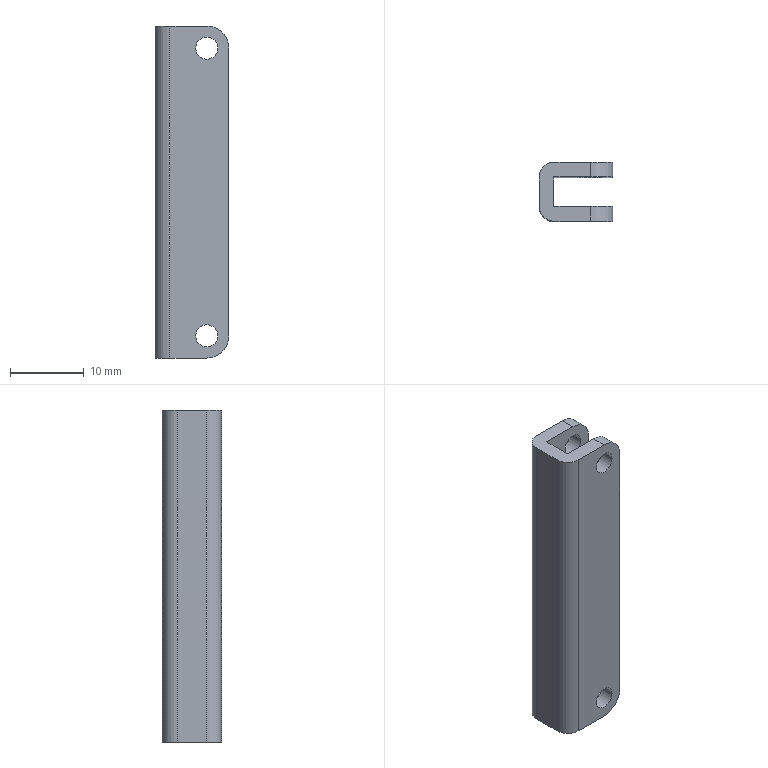Part | SolidWorks | features Extrusion 1, Fillet 1, ICE 1 | 1 solid | 24 faces | box 10 x 8 x 45 mm | volume 2011 mm3 | cylinder 14 | plane 10 | commonest cylinder face diameters 3 x8 6 x4 4 x2
STEP:
#1=CARTESIAN_POINT('',(-4.5,4.,3.));
#2=VERTEX_POINT('',#1);
#3=CARTESIAN_POINT('',(-1.5,4.,3.));
#4=VERTEX_POINT('',#3);
#5=CARTESIAN_POINT('',(-3.,4.,3.));
#6=DIRECTION('',(0.,-1.,0.));
#7=DIRECTION('',(1.,0.,0.));
#8=AXIS2_PLACEMENT_3D('',#5,#6,#7);
#9=CIRCLE('',#8,1.5);
#10=EDGE_CURVE('',#2,#4,#9,.T.);
#11=ORIENTED_EDGE('',*,*,#10,.F.);
#12=CARTESIAN_POINT('',(-4.5,2.,3.));
#13=VERTEX_POINT('',#12);
#14=CARTESIAN_POINT('',(-4.5,4.,3.));
#15=DIRECTION('',(0.,-1.,0.));
#16=VECTOR('',#15,1000.);
#17=LINE('',#14,#16);
#18=EDGE_CURVE('',#2,#13,#17,.T.);
#19=ORIENTED_EDGE('',*,*,#18,.T.);
#20=CARTESIAN_POINT('',(-1.5,2.,3.));
#21=VERTEX_POINT('',#20);
#22=CARTESIAN_POINT('',(-3.,2.,3.));
#23=DIRECTION('',(0.,1.,0.));
#24=DIRECTION('',(-1.,0.,0.));
#25=AXIS2_PLACEMENT_3D('',#22,#23,#24);
#26=CIRCLE('',#25,1.5);
#27=EDGE_CURVE('',#21,#13,#26,.T.);
#28=ORIENTED_EDGE('',*,*,#27,.F.);
#29=CARTESIAN_POINT('',(-1.5,4.,3.));
#30=DIRECTION('',(0.,-1.,0.));
#31=VECTOR('',#30,1000.);
#32=LINE('',#29,#31);
#33=EDGE_CURVE('',#4,#21,#32,.T.);
#34=ORIENTED_EDGE('',*,*,#33,.F.);
#35=EDGE_LOOP('',(#11,#19,#28,#34));
#36=FACE_OUTER_BOUND('',#35,.T.);
#37=CARTESIAN_POINT('',(-3.,4.,3.));
#38=DIRECTION('',(0.,-1.,0.));
#39=DIRECTION('',(1.,0.,0.));
#40=AXIS2_PLACEMENT_3D('',#37,#38,#39);
#41=CYLINDRICAL_SURFACE('',#40,1.5);
#42=ADVANCED_FACE('',(#36),#41,.F.);
#43=CARTESIAN_POINT('',(-4.5,4.,42.));
#44=VERTEX_POINT('',#43);
#45=CARTESIAN_POINT('',(-1.5,4.,42.));
#46=VERTEX_POINT('',#45);
#47=CARTESIAN_POINT('',(-3.,4.,42.));
#48=DIRECTION('',(0.,-1.,0.));
#49=DIRECTION('',(1.,0.,0.));
#50=AXIS2_PLACEMENT_3D('',#47,#48,#49);
#51=CIRCLE('',#50,1.5);
#52=EDGE_CURVE('',#44,#46,#51,.T.);
#53=ORIENTED_EDGE('',*,*,#52,.F.);
#54=CARTESIAN_POINT('',(-4.5,2.,42.));
#55=VERTEX_POINT('',#54);
#56=CARTESIAN_POINT('',(-4.5,4.,42.));
#57=DIRECTION('',(0.,-1.,0.));
#58=VECTOR('',#57,1000.);
#59=LINE('',#56,#58);
#60=EDGE_CURVE('',#44,#55,#59,.T.);
#61=ORIENTED_EDGE('',*,*,#60,.T.);
#62=CARTESIAN_POINT('',(-1.5,2.,42.));
#63=VERTEX_POINT('',#62);
#64=CARTESIAN_POINT('',(-3.,2.,42.));
#65=DIRECTION('',(0.,1.,0.));
#66=DIRECTION('',(-1.,0.,0.));
#67=AXIS2_PLACEMENT_3D('',#64,#65,#66);
#68=CIRCLE('',#67,1.5);
#69=EDGE_CURVE('',#63,#55,#68,.T.);
#70=ORIENTED_EDGE('',*,*,#69,.F.);
#71=CARTESIAN_POINT('',(-1.5,4.,42.));
#72=DIRECTION('',(0.,-1.,0.));
#73=VECTOR('',#72,1000.);
#74=LINE('',#71,#73);
#75=EDGE_CURVE('',#46,#63,#74,.T.);
#76=ORIENTED_EDGE('',*,*,#75,.F.);
#77=EDGE_LOOP('',(#53,#61,#70,#76));
#78=FACE_OUTER_BOUND('',#77,.T.);
#79=CARTESIAN_POINT('',(-3.,4.,42.));
#80=DIRECTION('',(0.,-1.,0.));
#81=DIRECTION('',(1.,0.,0.));
#82=AXIS2_PLACEMENT_3D('',#79,#80,#81);
#83=CYLINDRICAL_SURFACE('',#82,1.5);
#84=ADVANCED_FACE('',(#78),#83,.F.);
#85=CARTESIAN_POINT('',(-4.5,-2.,3.));
#86=VERTEX_POINT('',#85);
#87=CARTESIAN_POINT('',(-1.5,-2.,3.));
#88=VERTEX_POINT('',#87);
#89=CARTESIAN_POINT('',(-3.,-2.,3.));
#90=DIRECTION('',(0.,-1.,0.));
#91=DIRECTION('',(1.,0.,0.));
#92=AXIS2_PLACEMENT_3D('',#89,#90,#91);
#93=CIRCLE('',#92,1.5);
#94=EDGE_CURVE('',#86,#88,#93,.T.);
#95=ORIENTED_EDGE('',*,*,#94,.F.);
#96=CARTESIAN_POINT('',(-4.5,-4.,3.));
#97=VERTEX_POINT('',#96);
#98=CARTESIAN_POINT('',(-4.5,4.,3.));
#99=DIRECTION('',(0.,-1.,0.));
#100=VECTOR('',#99,1000.);
#101=LINE('',#98,#100);
#102=EDGE_CURVE('',#86,#97,#101,.T.);
#103=ORIENTED_EDGE('',*,*,#102,.T.);
#104=CARTESIAN_POINT('',(-1.5,-4.,3.));
#105=VERTEX_POINT('',#104);
#106=CARTESIAN_POINT('',(-3.,-4.,3.));
#107=DIRECTION('',(0.,-1.,0.));
#108=DIRECTION('',(1.,0.,0.));
#109=AXIS2_PLACEMENT_3D('',#106,#107,#108);
#110=CIRCLE('',#109,1.5);
#111=EDGE_CURVE('',#97,#105,#110,.T.);
#112=ORIENTED_EDGE('',*,*,#111,.T.);
#113=CARTESIAN_POINT('',(-1.5,4.,3.));
#114=DIRECTION('',(0.,-1.,0.));
#115=VECTOR('',#114,1000.);
#116=LINE('',#113,#115);
#117=EDGE_CURVE('',#88,#105,#116,.T.);
#118=ORIENTED_EDGE('',*,*,#117,.F.);
#119=EDGE_LOOP('',(#95,#103,#112,#118));
#120=FACE_OUTER_BOUND('',#119,.T.);
#121=CARTESIAN_POINT('',(-3.,4.,3.));
#122=DIRECTION('',(0.,-1.,0.));
#123=DIRECTION('',(1.,0.,0.));
#124=AXIS2_PLACEMENT_3D('',#121,#122,#123);
#125=CYLINDRICAL_SURFACE('',#124,1.5);
#126=ADVANCED_FACE('',(#120),#125,.F.);
#127=CARTESIAN_POINT('',(-4.5,-2.,42.));
#128=VERTEX_POINT('',#127);
#129=CARTESIAN_POINT('',(-1.5,-2.,42.));
#130=VERTEX_POINT('',#129);
#131=CARTESIAN_POINT('',(-3.,-2.,42.));
#132=DIRECTION('',(0.,-1.,0.));
#133=DIRECTION('',(1.,0.,0.));
#134=AXIS2_PLACEMENT_3D('',#131,#132,#133);
#135=CIRCLE('',#134,1.5);
#136=EDGE_CURVE('',#128,#130,#135,.T.);
#137=ORIENTED_EDGE('',*,*,#136,.F.);
#138=CARTESIAN_POINT('',(-4.5,-4.,42.));
#139=VERTEX_POINT('',#138);
#140=CARTESIAN_POINT('',(-4.5,4.,42.));
#141=DIRECTION('',(0.,-1.,0.));
#142=VECTOR('',#141,1000.);
#143=LINE('',#140,#142);
#144=EDGE_CURVE('',#128,#139,#143,.T.);
#145=ORIENTED_EDGE('',*,*,#144,.T.);
#146=CARTESIAN_POINT('',(-1.5,-4.,42.));
#147=VERTEX_POINT('',#146);
#148=CARTESIAN_POINT('',(-3.,-4.,42.));
#149=DIRECTION('',(0.,-1.,0.));
#150=DIRECTION('',(1.,0.,0.));
#151=AXIS2_PLACEMENT_3D('',#148,#149,#150);
#152=CIRCLE('',#151,1.5);
#153=EDGE_CURVE('',#139,#147,#152,.T.);
#154=ORIENTED_EDGE('',*,*,#153,.T.);
#155=CARTESIAN_POINT('',(-1.5,4.,42.));
#156=DIRECTION('',(0.,-1.,0.));
#157=VECTOR('',#156,1000.);
#158=LINE('',#155,#157);
#159=EDGE_CURVE('',#130,#147,#158,.T.);
#160=ORIENTED_EDGE('',*,*,#159,.F.);
#161=EDGE_LOOP('',(#137,#145,#154,#160));
#162=FACE_OUTER_BOUND('',#161,.T.);
#163=CARTESIAN_POINT('',(-3.,4.,42.));
#164=DIRECTION('',(0.,-1.,0.));
#165=DIRECTION('',(1.,0.,0.));
#166=AXIS2_PLACEMENT_3D('',#163,#164,#165);
#167=CYLINDRICAL_SURFACE('',#166,1.5);
#168=ADVANCED_FACE('',(#162),#167,.F.);
#169=CARTESIAN_POINT('',(0.,-2.,42.));
#170=VERTEX_POINT('',#169);
#171=CARTESIAN_POINT('',(0.,-2.,3.));
#172=VERTEX_POINT('',#171);
#173=CARTESIAN_POINT('',(0.,-2.,45.));
#174=DIRECTION('',(0.,0.,-1.));
#175=VECTOR('',#174,1000.);
#176=LINE('',#173,#175);
#177=EDGE_CURVE('',#170,#172,#176,.T.);
#178=ORIENTED_EDGE('',*,*,#177,.F.);
#179=CARTESIAN_POINT('',(0.,-4.,42.));
#180=VERTEX_POINT('',#179);
#181=CARTESIAN_POINT('',(0.,-4.,42.));
#182=DIRECTION('',(0.,-1.,0.));
#183=VECTOR('',#182,1000.);
#184=LINE('',#181,#183);
#185=EDGE_CURVE('',#170,#180,#184,.T.);
#186=ORIENTED_EDGE('',*,*,#185,.T.);
#187=CARTESIAN_POINT('',(0.,-4.,3.));
#188=VERTEX_POINT('',#187);
#189=CARTESIAN_POINT('',(0.,-4.,45.));
#190=DIRECTION('',(0.,0.,-1.));
#191=VECTOR('',#190,1000.);
#192=LINE('',#189,#191);
#193=EDGE_CURVE('',#180,#188,#192,.T.);
#194=ORIENTED_EDGE('',*,*,#193,.T.);
#195=CARTESIAN_POINT('',(0.,-4.,3.));
#196=DIRECTION('',(0.,1.,0.));
#197=VECTOR('',#196,1000.);
#198=LINE('',#195,#197);
#199=EDGE_CURVE('',#188,#172,#198,.T.);
#200=ORIENTED_EDGE('',*,*,#199,.T.);
#201=EDGE_LOOP('',(#178,#186,#194,#200));
#202=FACE_OUTER_BOUND('',#201,.T.);
#203=CARTESIAN_POINT('',(0.,-4.,45.));
#204=DIRECTION('',(-1.,0.,0.));
#205=DIRECTION('',(0.,-1.,0.));
#206=AXIS2_PLACEMENT_3D('',#203,#204,#205);
#207=PLANE('',#206);
#208=ADVANCED_FACE('',(#202),#207,.F.);
#209=CARTESIAN_POINT('',(-3.,-2.,3.));
#210=DIRECTION('',(0.,-1.,0.));
#211=DIRECTION('',(1.,0.,0.));
#212=AXIS2_PLACEMENT_3D('',#209,#210,#211);
#213=CIRCLE('',#212,1.5);
#214=EDGE_CURVE('',#88,#86,#213,.T.);
#215=ORIENTED_EDGE('',*,*,#214,.T.);
#216=ORIENTED_EDGE('',*,*,#94,.T.);
#217=EDGE_LOOP('',(#215,#216));
#218=FACE_BOUND('',#217,.T.);
#219=CARTESIAN_POINT('',(-3.,-2.,42.));
#220=DIRECTION('',(0.,-1.,0.));
#221=DIRECTION('',(1.,0.,0.));
#222=AXIS2_PLACEMENT_3D('',#219,#220,#221);
#223=CIRCLE('',#222,1.5);
#224=EDGE_CURVE('',#130,#128,#223,.T.);
#225=ORIENTED_EDGE('',*,*,#224,.T.);
#226=ORIENTED_EDGE('',*,*,#136,.T.);
#227=EDGE_LOOP('',(#225,#226));
#228=FACE_BOUND('',#227,.T.);
#229=CARTESIAN_POINT('',(-3.,-2.,45.));
#230=VERTEX_POINT('',#229);
#231=CARTESIAN_POINT('',(-8.,-2.,45.));
#232=VERTEX_POINT('',#231);
#233=CARTESIAN_POINT('',(-8.,-2.,45.));
#234=DIRECTION('',(-1.,0.,0.));
#235=VECTOR('',#234,1000.);
#236=LINE('',#233,#235);
#237=EDGE_CURVE('',#230,#232,#236,.T.);
#238=ORIENTED_EDGE('',*,*,#237,.F.);
#239=CARTESIAN_POINT('',(-3.,-2.,42.));
#240=DIRECTION('',(0.,1.,0.));
#241=DIRECTION('',(1.,0.,0.));
#242=AXIS2_PLACEMENT_3D('',#239,#240,#241);
#243=CIRCLE('',#242,3.);
#244=EDGE_CURVE('',#230,#170,#243,.T.);
#245=ORIENTED_EDGE('',*,*,#244,.T.);
#246=ORIENTED_EDGE('',*,*,#177,.T.);
#247=CARTESIAN_POINT('',(-3.,-2.,0.));
#248=VERTEX_POINT('',#247);
#249=CARTESIAN_POINT('',(-3.,-2.,3.));
#250=DIRECTION('',(0.,1.,0.));
#251=DIRECTION('',(1.,0.,0.));
#252=AXIS2_PLACEMENT_3D('',#249,#250,#251);
#253=CIRCLE('',#252,3.);
#254=EDGE_CURVE('',#172,#248,#253,.T.);
#255=ORIENTED_EDGE('',*,*,#254,.T.);
#256=CARTESIAN_POINT('',(-8.,-2.,0.));
#257=VERTEX_POINT('',#256);
#258=CARTESIAN_POINT('',(-8.,-2.,0.));
#259=DIRECTION('',(-1.,0.,0.));
#260=VECTOR('',#259,1000.);
#261=LINE('',#258,#260);
#262=EDGE_CURVE('',#248,#257,#261,.T.);
#263=ORIENTED_EDGE('',*,*,#262,.T.);
#264=CARTESIAN_POINT('',(-8.,-2.,45.));
#265=DIRECTION('',(0.,0.,-1.));
#266=VECTOR('',#265,1000.);
#267=LINE('',#264,#266);
#268=EDGE_CURVE('',#232,#257,#267,.T.);
#269=ORIENTED_EDGE('',*,*,#268,.F.);
#270=EDGE_LOOP('',(#238,#245,#246,#255,#263,#269));
#271=FACE_OUTER_BOUND('',#270,.T.);
#272=CARTESIAN_POINT('',(-8.,-2.,45.));
#273=DIRECTION('',(0.,-1.,0.));
#274=DIRECTION('',(1.,0.,0.));
#275=AXIS2_PLACEMENT_3D('',#272,#273,#274);
#276=PLANE('',#275);
#277=ADVANCED_FACE('',(#218,#228,#271),#276,.F.);
#278=CARTESIAN_POINT('',(-8.,2.,0.));
#279=VERTEX_POINT('',#278);
#280=CARTESIAN_POINT('',(-8.,2.,0.));
#281=DIRECTION('',(0.,1.,0.));
#282=VECTOR('',#281,1000.);
#283=LINE('',#280,#282);
#284=EDGE_CURVE('',#257,#279,#283,.T.);
#285=ORIENTED_EDGE('',*,*,#284,.T.);
#286=CARTESIAN_POINT('',(-8.,2.,45.));
#287=VERTEX_POINT('',#286);
#288=CARTESIAN_POINT('',(-8.,2.,45.));
#289=DIRECTION('',(0.,0.,-1.));
#290=VECTOR('',#289,1000.);
#291=LINE('',#288,#290);
#292=EDGE_CURVE('',#287,#279,#291,.T.);
#293=ORIENTED_EDGE('',*,*,#292,.F.);
#294=CARTESIAN_POINT('',(-8.,2.,45.));
#295=DIRECTION('',(0.,1.,0.));
#296=VECTOR('',#295,1000.);
#297=LINE('',#294,#296);
#298=EDGE_CURVE('',#232,#287,#297,.T.);
#299=ORIENTED_EDGE('',*,*,#298,.F.);
#300=ORIENTED_EDGE('',*,*,#268,.T.);
#301=EDGE_LOOP('',(#285,#293,#299,#300));
#302=FACE_OUTER_BOUND('',#301,.T.);
#303=CARTESIAN_POINT('',(-8.,2.,45.));
#304=DIRECTION('',(-1.,0.,0.));
#305=DIRECTION('',(0.,0.,1.));
#306=AXIS2_PLACEMENT_3D('',#303,#304,#305);
#307=PLANE('',#306);
#308=ADVANCED_FACE('',(#302),#307,.F.);
#309=ORIENTED_EDGE('',*,*,#27,.T.);
#310=CARTESIAN_POINT('',(-3.,2.,3.));
#311=DIRECTION('',(0.,1.,0.));
#312=DIRECTION('',(-1.,0.,0.));
#313=AXIS2_PLACEMENT_3D('',#310,#311,#312);
#314=CIRCLE('',#313,1.5);
#315=EDGE_CURVE('',#13,#21,#314,.T.);
#316=ORIENTED_EDGE('',*,*,#315,.T.);
#317=EDGE_LOOP('',(#309,#316));
#318=FACE_BOUND('',#317,.T.);
#319=ORIENTED_EDGE('',*,*,#69,.T.);
#320=CARTESIAN_POINT('',(-3.,2.,42.));
#321=DIRECTION('',(0.,1.,0.));
#322=DIRECTION('',(-1.,0.,0.));
#323=AXIS2_PLACEMENT_3D('',#320,#321,#322);
#324=CIRCLE('',#323,1.5);
#325=EDGE_CURVE('',#55,#63,#324,.T.);
#326=ORIENTED_EDGE('',*,*,#325,.T.);
#327=EDGE_LOOP('',(#319,#326));
#328=FACE_BOUND('',#327,.T.);
#329=CARTESIAN_POINT('',(0.,2.,42.));
#330=VERTEX_POINT('',#329);
#331=CARTESIAN_POINT('',(0.,2.,3.));
#332=VERTEX_POINT('',#331);
#333=CARTESIAN_POINT('',(0.,2.,45.));
#334=DIRECTION('',(0.,0.,-1.));
#335=VECTOR('',#334,1000.);
#336=LINE('',#333,#335);
#337=EDGE_CURVE('',#330,#332,#336,.T.);
#338=ORIENTED_EDGE('',*,*,#337,.F.);
#339=CARTESIAN_POINT('',(-3.,2.,45.));
#340=VERTEX_POINT('',#339);
#341=CARTESIAN_POINT('',(-3.,2.,42.));
#342=DIRECTION('',(0.,-1.,0.));
#343=DIRECTION('',(-1.,0.,0.));
#344=AXIS2_PLACEMENT_3D('',#341,#342,#343);
#345=CIRCLE('',#344,3.);
#346=EDGE_CURVE('',#330,#340,#345,.T.);
#347=ORIENTED_EDGE('',*,*,#346,.T.);
#348=CARTESIAN_POINT('',(-8.,2.,45.));
#349=DIRECTION('',(1.,0.,0.));
#350=VECTOR('',#349,1000.);
#351=LINE('',#348,#350);
#352=EDGE_CURVE('',#287,#340,#351,.T.);
#353=ORIENTED_EDGE('',*,*,#352,.F.);
#354=ORIENTED_EDGE('',*,*,#292,.T.);
#355=CARTESIAN_POINT('',(-3.,2.,0.));
#356=VERTEX_POINT('',#355);
#357=CARTESIAN_POINT('',(-8.,2.,0.));
#358=DIRECTION('',(1.,0.,0.));
#359=VECTOR('',#358,1000.);
#360=LINE('',#357,#359);
#361=EDGE_CURVE('',#279,#356,#360,.T.);
#362=ORIENTED_EDGE('',*,*,#361,.T.);
#363=CARTESIAN_POINT('',(-3.,2.,3.));
#364=DIRECTION('',(0.,-1.,0.));
#365=DIRECTION('',(-1.,0.,0.));
#366=AXIS2_PLACEMENT_3D('',#363,#364,#365);
#367=CIRCLE('',#366,3.);
#368=EDGE_CURVE('',#356,#332,#367,.T.);
#369=ORIENTED_EDGE('',*,*,#368,.T.);
#370=EDGE_LOOP('',(#338,#347,#353,#354,#362,#369));
#371=FACE_OUTER_BOUND('',#370,.T.);
#372=CARTESIAN_POINT('',(-8.,2.,45.));
#373=DIRECTION('',(0.,1.,0.));
#374=DIRECTION('',(-1.,0.,0.));
#375=AXIS2_PLACEMENT_3D('',#372,#373,#374);
#376=PLANE('',#375);
#377=ADVANCED_FACE('',(#318,#328,#371),#376,.F.);
#378=CARTESIAN_POINT('',(0.,4.,42.));
#379=VERTEX_POINT('',#378);
#380=CARTESIAN_POINT('',(0.,4.,3.));
#381=VERTEX_POINT('',#380);
#382=CARTESIAN_POINT('',(0.,4.,45.));
#383=DIRECTION('',(0.,0.,-1.));
#384=VECTOR('',#383,1000.);
#385=LINE('',#382,#384);
#386=EDGE_CURVE('',#379,#381,#385,.T.);
#387=ORIENTED_EDGE('',*,*,#386,.F.);
#388=CARTESIAN_POINT('',(0.,2.,42.));
#389=DIRECTION('',(0.,-1.,0.));
#390=VECTOR('',#389,1000.);
#391=LINE('',#388,#390);
#392=EDGE_CURVE('',#379,#330,#391,.T.);
#393=ORIENTED_EDGE('',*,*,#392,.T.);
#394=ORIENTED_EDGE('',*,*,#337,.T.);
#395=CARTESIAN_POINT('',(0.,4.,3.));
#396=DIRECTION('',(0.,1.,0.));
#397=VECTOR('',#396,1000.);
#398=LINE('',#395,#397);
#399=EDGE_CURVE('',#332,#381,#398,.T.);
#400=ORIENTED_EDGE('',*,*,#399,.T.);
#401=EDGE_LOOP('',(#387,#393,#394,#400));
#402=FACE_OUTER_BOUND('',#401,.T.);
#403=CARTESIAN_POINT('',(0.,4.,45.));
#404=DIRECTION('',(-1.,0.,0.));
#405=DIRECTION('',(0.,-1.,0.));
#406=AXIS2_PLACEMENT_3D('',#403,#404,#405);
#407=PLANE('',#406);
#408=ADVANCED_FACE('',(#402),#407,.F.);
#409=CARTESIAN_POINT('',(-3.,4.,3.));
#410=DIRECTION('',(0.,-1.,0.));
#411=DIRECTION('',(1.,0.,0.));
#412=AXIS2_PLACEMENT_3D('',#409,#410,#411);
#413=CIRCLE('',#412,1.5);
#414=EDGE_CURVE('',#4,#2,#413,.T.);
#415=ORIENTED_EDGE('',*,*,#414,.T.);
#416=ORIENTED_EDGE('',*,*,#10,.T.);
#417=EDGE_LOOP('',(#415,#416));
#418=FACE_BOUND('',#417,.T.);
#419=CARTESIAN_POINT('',(-3.,4.,42.));
#420=DIRECTION('',(0.,-1.,0.));
#421=DIRECTION('',(1.,0.,0.));
#422=AXIS2_PLACEMENT_3D('',#419,#420,#421);
#423=CIRCLE('',#422,1.5);
#424=EDGE_CURVE('',#46,#44,#423,.T.);
#425=ORIENTED_EDGE('',*,*,#424,.T.);
#426=ORIENTED_EDGE('',*,*,#52,.T.);
#427=EDGE_LOOP('',(#425,#426));
#428=FACE_BOUND('',#427,.T.);
#429=CARTESIAN_POINT('',(-3.,4.,45.));
#430=VERTEX_POINT('',#429);
#431=CARTESIAN_POINT('',(-8.,4.,45.));
#432=VERTEX_POINT('',#431);
#433=CARTESIAN_POINT('',(-8.,4.,45.));
#434=DIRECTION('',(-1.,0.,0.));
#435=VECTOR('',#434,1000.);
#436=LINE('',#433,#435);
#437=EDGE_CURVE('',#430,#432,#436,.T.);
#438=ORIENTED_EDGE('',*,*,#437,.F.);
#439=CARTESIAN_POINT('',(-3.,4.,42.));
#440=DIRECTION('',(0.,1.,0.));
#441=DIRECTION('',(1.,0.,0.));
#442=AXIS2_PLACEMENT_3D('',#439,#440,#441);
#443=CIRCLE('',#442,3.);
#444=EDGE_CURVE('',#430,#379,#443,.T.);
#445=ORIENTED_EDGE('',*,*,#444,.T.);
#446=ORIENTED_EDGE('',*,*,#386,.T.);
#447=CARTESIAN_POINT('',(-3.,4.,0.));
#448=VERTEX_POINT('',#447);
#449=CARTESIAN_POINT('',(-3.,4.,3.));
#450=DIRECTION('',(0.,1.,0.));
#451=DIRECTION('',(1.,0.,0.));
#452=AXIS2_PLACEMENT_3D('',#449,#450,#451);
#453=CIRCLE('',#452,3.);
#454=EDGE_CURVE('',#381,#448,#453,.T.);
#455=ORIENTED_EDGE('',*,*,#454,.T.);
#456=CARTESIAN_POINT('',(-8.,4.,0.));
#457=VERTEX_POINT('',#456);
#458=CARTESIAN_POINT('',(-8.,4.,0.));
#459=DIRECTION('',(-1.,0.,0.));
#460=VECTOR('',#459,1000.);
#461=LINE('',#458,#460);
#462=EDGE_CURVE('',#448,#457,#461,.T.);
#463=ORIENTED_EDGE('',*,*,#462,.T.);
#464=CARTESIAN_POINT('',(-8.,4.,45.));
#465=DIRECTION('',(0.,0.,-1.));
#466=VECTOR('',#465,1000.);
#467=LINE('',#464,#466);
#468=EDGE_CURVE('',#432,#457,#467,.T.);
#469=ORIENTED_EDGE('',*,*,#468,.F.);
#470=EDGE_LOOP('',(#438,#445,#446,#455,#463,#469));
#471=FACE_OUTER_BOUND('',#470,.T.);
#472=CARTESIAN_POINT('',(-8.,4.,45.));
#473=DIRECTION('',(0.,-1.,0.));
#474=DIRECTION('',(1.,0.,0.));
#475=AXIS2_PLACEMENT_3D('',#472,#473,#474);
#476=PLANE('',#475);
#477=ADVANCED_FACE('',(#418,#428,#471),#476,.F.);
#478=CARTESIAN_POINT('',(-10.,2.,0.));
#479=VERTEX_POINT('',#478);
#480=CARTESIAN_POINT('',(-8.,2.,0.));
#481=DIRECTION('',(0.,0.,1.));
#482=DIRECTION('',(1.,0.,0.));
#483=AXIS2_PLACEMENT_3D('',#480,#481,#482);
#484=CIRCLE('',#483,2.);
#485=EDGE_CURVE('',#457,#479,#484,.T.);
#486=ORIENTED_EDGE('',*,*,#485,.T.);
#487=CARTESIAN_POINT('',(-10.,2.,45.));
#488=VERTEX_POINT('',#487);
#489=CARTESIAN_POINT('',(-10.,2.,45.));
#490=DIRECTION('',(0.,0.,-1.));
#491=VECTOR('',#490,1000.);
#492=LINE('',#489,#491);
#493=EDGE_CURVE('',#488,#479,#492,.T.);
#494=ORIENTED_EDGE('',*,*,#493,.F.);
#495=CARTESIAN_POINT('',(-8.,2.,45.));
#496=DIRECTION('',(0.,0.,1.));
#497=DIRECTION('',(1.,0.,0.));
#498=AXIS2_PLACEMENT_3D('',#495,#496,#497);
#499=CIRCLE('',#498,2.);
#500=EDGE_CURVE('',#432,#488,#499,.T.);
#501=ORIENTED_EDGE('',*,*,#500,.F.);
#502=ORIENTED_EDGE('',*,*,#468,.T.);
#503=EDGE_LOOP('',(#486,#494,#501,#502));
#504=FACE_OUTER_BOUND('',#503,.T.);
#505=CARTESIAN_POINT('',(-8.,2.,45.));
#506=DIRECTION('',(0.,0.,-1.));
#507=DIRECTION('',(-1.,0.,0.));
#508=AXIS2_PLACEMENT_3D('',#505,#506,#507);
#509=CYLINDRICAL_SURFACE('',#508,2.);
#510=ADVANCED_FACE('',(#504),#509,.T.);
#511=CARTESIAN_POINT('',(-10.,-2.,0.));
#512=VERTEX_POINT('',#511);
#513=CARTESIAN_POINT('',(-10.,2.,0.));
#514=DIRECTION('',(0.,-1.,0.));
#515=VECTOR('',#514,1000.);
#516=LINE('',#513,#515);
#517=EDGE_CURVE('',#479,#512,#516,.T.);
#518=ORIENTED_EDGE('',*,*,#517,.T.);
#519=CARTESIAN_POINT('',(-10.,-2.,45.));
#520=VERTEX_POINT('',#519);
#521=CARTESIAN_POINT('',(-10.,-2.,45.));
#522=DIRECTION('',(0.,0.,-1.));
#523=VECTOR('',#522,1000.);
#524=LINE('',#521,#523);
#525=EDGE_CURVE('',#520,#512,#524,.T.);
#526=ORIENTED_EDGE('',*,*,#525,.F.);
#527=CARTESIAN_POINT('',(-10.,2.,45.));
#528=DIRECTION('',(0.,-1.,0.));
#529=VECTOR('',#528,1000.);
#530=LINE('',#527,#529);
#531=EDGE_CURVE('',#488,#520,#530,.T.);
#532=ORIENTED_EDGE('',*,*,#531,.F.);
#533=ORIENTED_EDGE('',*,*,#493,.T.);
#534=EDGE_LOOP('',(#518,#526,#532,#533));
#535=FACE_OUTER_BOUND('',#534,.T.);
#536=CARTESIAN_POINT('',(-10.,2.,45.));
#537=DIRECTION('',(1.,0.,0.));
#538=DIRECTION('',(0.,0.,-1.));
#539=AXIS2_PLACEMENT_3D('',#536,#537,#538);
#540=PLANE('',#539);
#541=ADVANCED_FACE('',(#535),#540,.F.);
#542=CARTESIAN_POINT('',(-8.,-4.,0.));
#543=VERTEX_POINT('',#542);
#544=CARTESIAN_POINT('',(-8.,-2.,0.));
#545=DIRECTION('',(0.,0.,1.));
#546=DIRECTION('',(1.,0.,0.));
#547=AXIS2_PLACEMENT_3D('',#544,#545,#546);
#548=CIRCLE('',#547,2.);
#549=EDGE_CURVE('',#512,#543,#548,.T.);
#550=ORIENTED_EDGE('',*,*,#549,.T.);
#551=CARTESIAN_POINT('',(-8.,-4.,45.));
#552=VERTEX_POINT('',#551);
#553=CARTESIAN_POINT('',(-8.,-4.,45.));
#554=DIRECTION('',(0.,0.,-1.));
#555=VECTOR('',#554,1000.);
#556=LINE('',#553,#555);
#557=EDGE_CURVE('',#552,#543,#556,.T.);
#558=ORIENTED_EDGE('',*,*,#557,.F.);
#559=CARTESIAN_POINT('',(-8.,-2.,45.));
#560=DIRECTION('',(0.,0.,1.));
#561=DIRECTION('',(1.,0.,0.));
#562=AXIS2_PLACEMENT_3D('',#559,#560,#561);
#563=CIRCLE('',#562,2.);
#564=EDGE_CURVE('',#520,#552,#563,.T.);
#565=ORIENTED_EDGE('',*,*,#564,.F.);
#566=ORIENTED_EDGE('',*,*,#525,.T.);
#567=EDGE_LOOP('',(#550,#558,#565,#566));
#568=FACE_OUTER_BOUND('',#567,.T.);
#569=CARTESIAN_POINT('',(-8.,-2.,45.));
#570=DIRECTION('',(0.,0.,-1.));
#571=DIRECTION('',(-1.,0.,0.));
#572=AXIS2_PLACEMENT_3D('',#569,#570,#571);
#573=CYLINDRICAL_SURFACE('',#572,2.);
#574=ADVANCED_FACE('',(#568),#573,.T.);
#575=CARTESIAN_POINT('',(-3.,-4.,3.));
#576=DIRECTION('',(0.,-1.,0.));
#577=DIRECTION('',(1.,0.,0.));
#578=AXIS2_PLACEMENT_3D('',#575,#576,#577);
#579=CIRCLE('',#578,1.5);
#580=EDGE_CURVE('',#105,#97,#579,.T.);
#581=ORIENTED_EDGE('',*,*,#580,.F.);
#582=ORIENTED_EDGE('',*,*,#111,.F.);
#583=EDGE_LOOP('',(#581,#582));
#584=FACE_BOUND('',#583,.T.);
#585=CARTESIAN_POINT('',(-3.,-4.,42.));
#586=DIRECTION('',(0.,-1.,0.));
#587=DIRECTION('',(1.,0.,0.));
#588=AXIS2_PLACEMENT_3D('',#585,#586,#587);
#589=CIRCLE('',#588,1.5);
#590=EDGE_CURVE('',#147,#139,#589,.T.);
#591=ORIENTED_EDGE('',*,*,#590,.F.);
#592=ORIENTED_EDGE('',*,*,#153,.F.);
#593=EDGE_LOOP('',(#591,#592));
#594=FACE_BOUND('',#593,.T.);
#595=ORIENTED_EDGE('',*,*,#193,.F.);
#596=CARTESIAN_POINT('',(-3.,-4.,45.));
#597=VERTEX_POINT('',#596);
#598=CARTESIAN_POINT('',(-3.,-4.,42.));
#599=DIRECTION('',(0.,-1.,0.));
#600=DIRECTION('',(-1.,0.,0.));
#601=AXIS2_PLACEMENT_3D('',#598,#599,#600);
#602=CIRCLE('',#601,3.);
#603=EDGE_CURVE('',#180,#597,#602,.T.);
#604=ORIENTED_EDGE('',*,*,#603,.T.);
#605=CARTESIAN_POINT('',(-8.,-4.,45.));
#606=DIRECTION('',(1.,0.,0.));
#607=VECTOR('',#606,1000.);
#608=LINE('',#605,#607);
#609=EDGE_CURVE('',#552,#597,#608,.T.);
#610=ORIENTED_EDGE('',*,*,#609,.F.);
#611=ORIENTED_EDGE('',*,*,#557,.T.);
#612=CARTESIAN_POINT('',(-3.,-4.,0.));
#613=VERTEX_POINT('',#612);
#614=CARTESIAN_POINT('',(-8.,-4.,0.));
#615=DIRECTION('',(1.,0.,0.));
#616=VECTOR('',#615,1000.);
#617=LINE('',#614,#616);
#618=EDGE_CURVE('',#543,#613,#617,.T.);
#619=ORIENTED_EDGE('',*,*,#618,.T.);
#620=CARTESIAN_POINT('',(-3.,-4.,3.));
#621=DIRECTION('',(0.,-1.,0.));
#622=DIRECTION('',(-1.,0.,0.));
#623=AXIS2_PLACEMENT_3D('',#620,#621,#622);
#624=CIRCLE('',#623,3.);
#625=EDGE_CURVE('',#613,#188,#624,.T.);
#626=ORIENTED_EDGE('',*,*,#625,.T.);
#627=EDGE_LOOP('',(#595,#604,#610,#611,#619,#626));
#628=FACE_OUTER_BOUND('',#627,.T.);
#629=CARTESIAN_POINT('',(-8.,-4.,45.));
#630=DIRECTION('',(0.,1.,0.));
#631=DIRECTION('',(-1.,0.,0.));
#632=AXIS2_PLACEMENT_3D('',#629,#630,#631);
#633=PLANE('',#632);
#634=ADVANCED_FACE('',(#584,#594,#628),#633,.F.);
#635=ORIENTED_EDGE('',*,*,#352,.T.);
#636=CARTESIAN_POINT('',(-3.,4.,45.));
#637=DIRECTION('',(0.,1.,0.));
#638=VECTOR('',#637,1000.);
#639=LINE('',#636,#638);
#640=EDGE_CURVE('',#340,#430,#639,.T.);
#641=ORIENTED_EDGE('',*,*,#640,.T.);
#642=ORIENTED_EDGE('',*,*,#437,.T.);
#643=ORIENTED_EDGE('',*,*,#500,.T.);
#644=ORIENTED_EDGE('',*,*,#531,.T.);
#645=ORIENTED_EDGE('',*,*,#564,.T.);
#646=ORIENTED_EDGE('',*,*,#609,.T.);
#647=CARTESIAN_POINT('',(-3.,-2.,45.));
#648=DIRECTION('',(0.,1.,0.));
#649=VECTOR('',#648,1000.);
#650=LINE('',#647,#649);
#651=EDGE_CURVE('',#597,#230,#650,.T.);
#652=ORIENTED_EDGE('',*,*,#651,.T.);
#653=ORIENTED_EDGE('',*,*,#237,.T.);
#654=ORIENTED_EDGE('',*,*,#298,.T.);
#655=EDGE_LOOP('',(#635,#641,#642,#643,#644,#645,#646,#652,#653,#654));
#656=FACE_OUTER_BOUND('',#655,.T.);
#657=CARTESIAN_POINT('',(-8.,2.,45.));
#658=DIRECTION('',(0.,0.,1.));
#659=DIRECTION('',(1.,0.,0.));
#660=AXIS2_PLACEMENT_3D('',#657,#658,#659);
#661=PLANE('',#660);
#662=ADVANCED_FACE('',(#656),#661,.T.);
#663=ORIENTED_EDGE('',*,*,#262,.F.);
#664=CARTESIAN_POINT('',(-3.,2.,0.));
#665=DIRECTION('',(0.,-1.,0.));
#666=VECTOR('',#665,1000.);
#667=LINE('',#664,#666);
#668=EDGE_CURVE('',#248,#613,#667,.T.);
#669=ORIENTED_EDGE('',*,*,#668,.T.);
#670=ORIENTED_EDGE('',*,*,#618,.F.);
#671=ORIENTED_EDGE('',*,*,#549,.F.);
#672=ORIENTED_EDGE('',*,*,#517,.F.);
#673=ORIENTED_EDGE('',*,*,#485,.F.);
#674=ORIENTED_EDGE('',*,*,#462,.F.);
#675=CARTESIAN_POINT('',(-3.,2.,0.));
#676=DIRECTION('',(0.,-1.,0.));
#677=VECTOR('',#676,1000.);
#678=LINE('',#675,#677);
#679=EDGE_CURVE('',#448,#356,#678,.T.);
#680=ORIENTED_EDGE('',*,*,#679,.T.);
#681=ORIENTED_EDGE('',*,*,#361,.F.);
#682=ORIENTED_EDGE('',*,*,#284,.F.);
#683=EDGE_LOOP('',(#663,#669,#670,#671,#672,#673,#674,#680,#681,#682));
#684=FACE_OUTER_BOUND('',#683,.T.);
#685=CARTESIAN_POINT('',(-8.,2.,0.));
#686=DIRECTION('',(0.,0.,1.));
#687=DIRECTION('',(1.,0.,0.));
#688=AXIS2_PLACEMENT_3D('',#685,#686,#687);
#689=PLANE('',#688);
#690=ADVANCED_FACE('',(#684),#689,.F.);
#691=ORIENTED_EDGE('',*,*,#144,.F.);
#692=ORIENTED_EDGE('',*,*,#224,.F.);
#693=ORIENTED_EDGE('',*,*,#159,.T.);
#694=ORIENTED_EDGE('',*,*,#590,.T.);
#695=EDGE_LOOP('',(#691,#692,#693,#694));
#696=FACE_OUTER_BOUND('',#695,.T.);
#697=CARTESIAN_POINT('',(-3.,4.,42.));
#698=DIRECTION('',(0.,-1.,0.));
#699=DIRECTION('',(1.,0.,0.));
#700=AXIS2_PLACEMENT_3D('',#697,#698,#699);
#701=CYLINDRICAL_SURFACE('',#700,1.5);
#702=ADVANCED_FACE('',(#696),#701,.F.);
#703=ORIENTED_EDGE('',*,*,#102,.F.);
#704=ORIENTED_EDGE('',*,*,#214,.F.);
#705=ORIENTED_EDGE('',*,*,#117,.T.);
#706=ORIENTED_EDGE('',*,*,#580,.T.);
#707=EDGE_LOOP('',(#703,#704,#705,#706));
#708=FACE_OUTER_BOUND('',#707,.T.);
#709=CARTESIAN_POINT('',(-3.,4.,3.));
#710=DIRECTION('',(0.,-1.,0.));
#711=DIRECTION('',(1.,0.,0.));
#712=AXIS2_PLACEMENT_3D('',#709,#710,#711);
#713=CYLINDRICAL_SURFACE('',#712,1.5);
#714=ADVANCED_FACE('',(#708),#713,.F.);
#715=ORIENTED_EDGE('',*,*,#60,.F.);
#716=ORIENTED_EDGE('',*,*,#424,.F.);
#717=ORIENTED_EDGE('',*,*,#75,.T.);
#718=ORIENTED_EDGE('',*,*,#325,.F.);
#719=EDGE_LOOP('',(#715,#716,#717,#718));
#720=FACE_OUTER_BOUND('',#719,.T.);
#721=CARTESIAN_POINT('',(-3.,4.,42.));
#722=DIRECTION('',(0.,-1.,0.));
#723=DIRECTION('',(1.,0.,0.));
#724=AXIS2_PLACEMENT_3D('',#721,#722,#723);
#725=CYLINDRICAL_SURFACE('',#724,1.5);
#726=ADVANCED_FACE('',(#720),#725,.F.);
#727=ORIENTED_EDGE('',*,*,#18,.F.);
#728=ORIENTED_EDGE('',*,*,#414,.F.);
#729=ORIENTED_EDGE('',*,*,#33,.T.);
#730=ORIENTED_EDGE('',*,*,#315,.F.);
#731=EDGE_LOOP('',(#727,#728,#729,#730));
#732=FACE_OUTER_BOUND('',#731,.T.);
#733=CARTESIAN_POINT('',(-3.,4.,3.));
#734=DIRECTION('',(0.,-1.,0.));
#735=DIRECTION('',(1.,0.,0.));
#736=AXIS2_PLACEMENT_3D('',#733,#734,#735);
#737=CYLINDRICAL_SURFACE('',#736,1.5);
#738=ADVANCED_FACE('',(#732),#737,.F.);
#739=ORIENTED_EDGE('',*,*,#346,.F.);
#740=ORIENTED_EDGE('',*,*,#392,.F.);
#741=ORIENTED_EDGE('',*,*,#444,.F.);
#742=ORIENTED_EDGE('',*,*,#640,.F.);
#743=EDGE_LOOP('',(#739,#740,#741,#742));
#744=FACE_OUTER_BOUND('',#743,.T.);
#745=CARTESIAN_POINT('',(-3.,2.,42.));
#746=DIRECTION('',(0.,-1.,0.));
#747=DIRECTION('',(1.,0.,0.));
#748=AXIS2_PLACEMENT_3D('',#745,#746,#747);
#749=CYLINDRICAL_SURFACE('',#748,3.);
#750=ADVANCED_FACE('',(#744),#749,.T.);
#751=ORIENTED_EDGE('',*,*,#603,.F.);
#752=ORIENTED_EDGE('',*,*,#185,.F.);
#753=ORIENTED_EDGE('',*,*,#244,.F.);
#754=ORIENTED_EDGE('',*,*,#651,.F.);
#755=EDGE_LOOP('',(#751,#752,#753,#754));
#756=FACE_OUTER_BOUND('',#755,.T.);
#757=CARTESIAN_POINT('',(-3.,2.,42.));
#758=DIRECTION('',(0.,-1.,0.));
#759=DIRECTION('',(1.,0.,0.));
#760=AXIS2_PLACEMENT_3D('',#757,#758,#759);
#761=CYLINDRICAL_SURFACE('',#760,3.);
#762=ADVANCED_FACE('',(#756),#761,.T.);
#763=ORIENTED_EDGE('',*,*,#625,.F.);
#764=ORIENTED_EDGE('',*,*,#668,.F.);
#765=ORIENTED_EDGE('',*,*,#254,.F.);
#766=ORIENTED_EDGE('',*,*,#199,.F.);
#767=EDGE_LOOP('',(#763,#764,#765,#766));
#768=FACE_OUTER_BOUND('',#767,.T.);
#769=CARTESIAN_POINT('',(-3.,-4.,3.));
#770=DIRECTION('',(0.,1.,0.));
#771=DIRECTION('',(-1.,0.,0.));
#772=AXIS2_PLACEMENT_3D('',#769,#770,#771);
#773=CYLINDRICAL_SURFACE('',#772,3.);
#774=ADVANCED_FACE('',(#768),#773,.T.);
#775=ORIENTED_EDGE('',*,*,#368,.F.);
#776=ORIENTED_EDGE('',*,*,#679,.F.);
#777=ORIENTED_EDGE('',*,*,#454,.F.);
#778=ORIENTED_EDGE('',*,*,#399,.F.);
#779=EDGE_LOOP('',(#775,#776,#777,#778));
#780=FACE_OUTER_BOUND('',#779,.T.);
#781=CARTESIAN_POINT('',(-3.,4.,3.));
#782=DIRECTION('',(0.,1.,0.));
#783=DIRECTION('',(-1.,0.,0.));
#784=AXIS2_PLACEMENT_3D('',#781,#782,#783);
#785=CYLINDRICAL_SURFACE('',#784,3.);
#786=ADVANCED_FACE('',(#780),#785,.T.);
#787=CLOSED_SHELL('',(#42,#84,#126,#168,#208,#277,#308,#377,#408,#477,#510,#541,#574,#634,#662,#690,#702,#714,#726,#738,#750,#762,#774,#786));
#788=MANIFOLD_SOLID_BREP('',#787);
#789=CARTESIAN_POINT('',(0.,0.,0.));
#790=DIRECTION('',(0.,0.,1.));
#791=DIRECTION('',(1.,0.,0.));
#792=AXIS2_PLACEMENT_3D('',#789,#790,#791);
#793=(LENGTH_UNIT()NAMED_UNIT(*)SI_UNIT(.MILLI.,.METRE.));
#794=UNCERTAINTY_MEASURE_WITH_UNIT(LENGTH_MEASURE(0.00001),#793,'','');
#795=(NAMED_UNIT(*)PLANE_ANGLE_UNIT()SI_UNIT($,.RADIAN.));
#796=(NAMED_UNIT(*)SI_UNIT($,.STERADIAN.)SOLID_ANGLE_UNIT());
#797=(GEOMETRIC_REPRESENTATION_CONTEXT(3)GLOBAL_UNCERTAINTY_ASSIGNED_CONTEXT((#794))GLOBAL_UNIT_ASSIGNED_CONTEXT((#793,#795,#796))REPRESENTATION_CONTEXT('',''));
#798=ADVANCED_BREP_SHAPE_REPRESENTATION('',(#788,#792),#797);